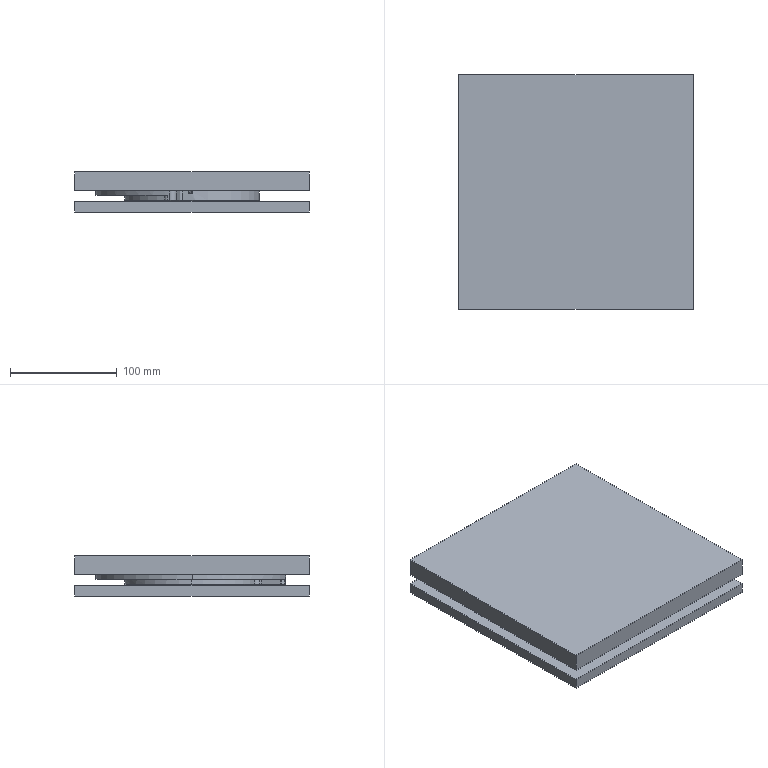NC program | NX | posted with a generic post | part box 220 x 220 x 37.5 mm
Lines 1 to 75 of 13716:
N10 G17 G21 G94 G90
(DRILLING_COPY_1 , TOOL : D6A45)
N12 T18 M6
N14 G54
N16 G17 G0 G90 X47. Y46. S3000 M3
N18 G43 Z30. H18
N20 G94 G81 G98 Z-1.55 F200. R3.
N22 Y36.
N24 G80
N26 G0 X47. Y36. Z30.
(DRILLING_COPY_1_COPY , TOOL : D6A45)
N28 X74.114 Y-22.659
N30 G81 Z-2.6 F200. R3.
N32 X75.514 Y17.434
N34 X56.68 Y52.855
N36 X36. Y38.5
N38 X22.659 Y74.114
N40 X-35.184 Y69.053
N42 X-71.857 Y29.032
N44 X-52.237 Y-5.25
N46 G80
N48 G0 X-52.237 Y-5.25 Z30.
N50 M5
(DRILLING_COPY_1_COPY_1 , TOOL : 2.6ZT)
N52 T12 M6
N54 G54
N56 G17 G0 G90 X47. Y46. S3000 M3
N58 G43 Z30. H12
N60 G94 G83 G98 Z-8.251 F120. Q2. R3.
N62 Y36.
N64 G80
N66 G0 X47. Y36. Z30.
N68 M5
(DRILLING_COPY_1_COPY_1_COPY_1 , TOOL : 5.2ZT)
N70 T15 M6
N72 G54
N74 G17 G0 G90 X74.114 Y-22.659 S3000 M3
N76 G43 Z30. H15
N78 G94 G83 G98 Z-15.002 F300. Q2. R3.
N80 X75.514 Y17.434
N82 X56.68 Y52.855
N84 X22.659 Y74.114
N86 X-35.184 Y69.053
N88 X-71.857 Y29.032
N90 G80
N92 G0 X-71.857 Y29.032 Z30.
(DRILLING_COPY_1_COPY_1_COPY_1_COPY_2 , TOOL : 5.2ZT)
N94 X36. Y38.5
N96 G83 Z-20.002 F300. Q2. R3.
N98 G80
N100 G0 X36. Y38.5 Z30.
N102 M5
(DRILLING_COPY_1_COPY_1_COPY_1_COPY_1 , TOOL : 4.5ZT)
N104 T14 M6
N106 G54
N108 G17 G0 G90 X-52.237 Y-5.25 S3000 M3
N110 G43 Z30. H14
N112 G94 G83 G98 Z-19.852 F300. Q2. R3.
N114 G80
N116 G0 X-52.237 Y-5.25 Z30.
N118 M5